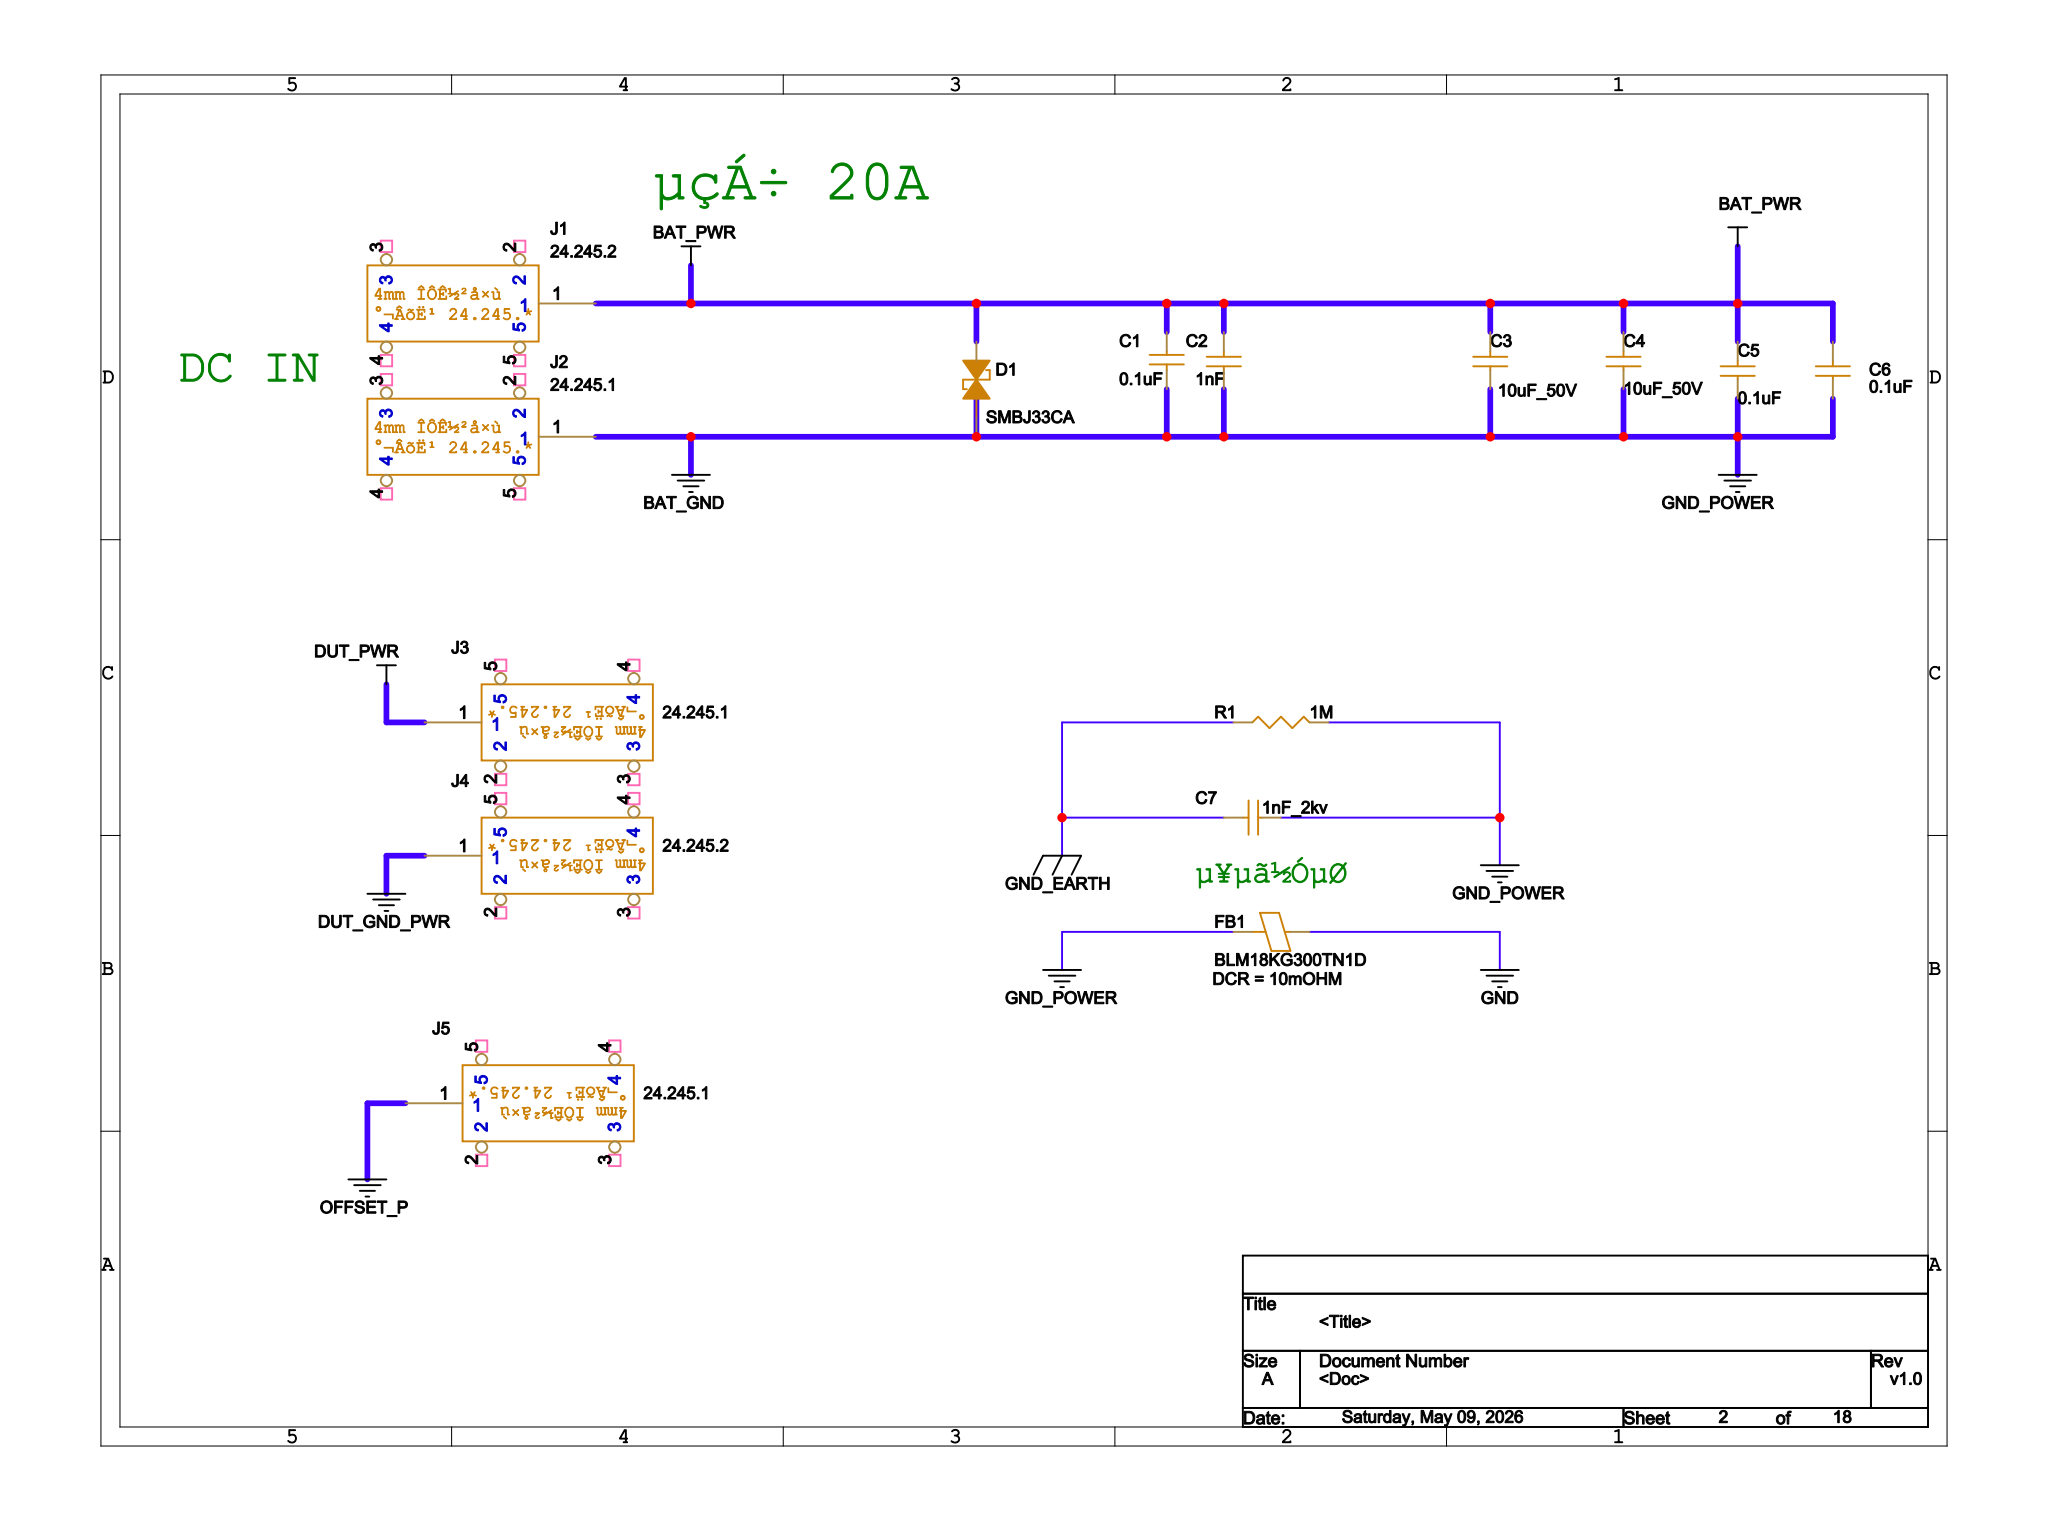Circuit board | Cadence Allegro | 330 parts | 215 nets | one sheet of the schematic
Parts on this sheet (reference | value | footprint):
C1 | 0.1uF | 0402
C2 | 1nF | 0402
C3 | 10uF_50V | 1210
C4 | 10uF_50V | 1210
C5 | 0.1uF | 0402
C6 | 0.1uF | 0402
C7 | 1nF_2kv | 1206
D1 | SMBJ33CA | DO-214AA
FB1 | BLM18KG300TN1D | 0603
J1 | 24.245.2 | C7437326
J2 | 24.245.1 | C7437326
J3 | 24.245.1 | C7437326
J4 | 24.245.2 | C7437326
J5 | 24.245.1 | C7437326
R1 | 1M | 1206
Nets of these parts (net: part-pin ...):
GND: FB1-1
BAT_GND: C1-2 C2-1 C3-1 C4-1 C5-1 C6-1 C7-1 D1-2 FB1-2 J2-1 R1-2
BAT_PWR: C1-1 C2-2 C3-2 C4-2 C5-2 C6-2 D1-1 J1-1
DUT_GND_PWR: J4-1
DUT_PWR: J3-1
OFFSET_P: J5-1
GND_EARTH: C7-2 R1-1